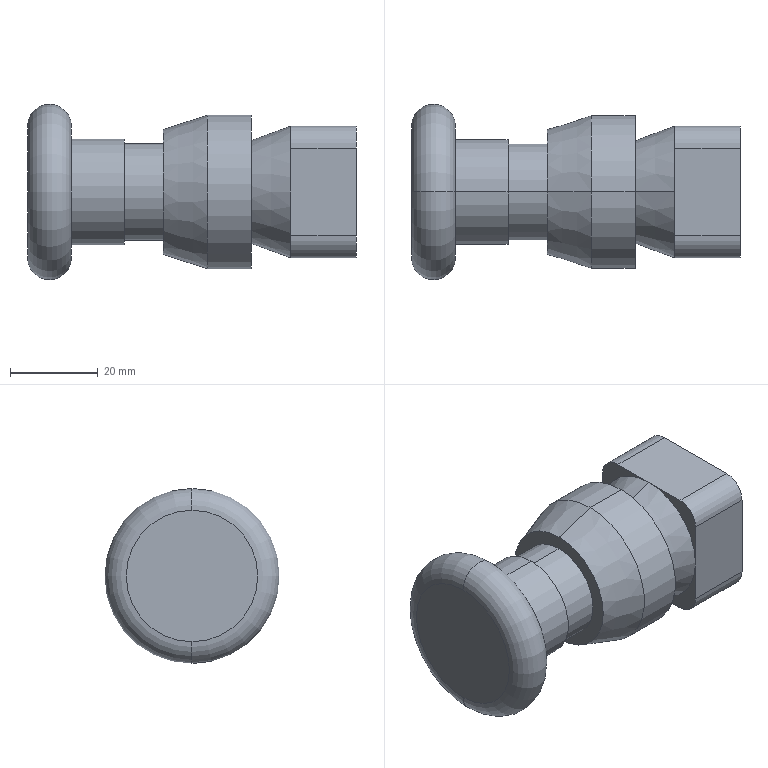Part | SolidWorks | features BaseBody 1 | 1 solid | 30 faces | box 75 x 40 x 40 mm | volume 55961 mm3 | plane 14 | cylinder 10 | cone 4 | torus 2 | commonest cylinder face diameters 10 x4 22 x2 24 x2 35 x2
STEP:
#1=CARTESIAN_POINT('',(3.054,-15.123,17.5));
#2=VERTEX_POINT('',#1);
#3=CARTESIAN_POINT('',(3.054,-15.123,-17.5));
#4=VERTEX_POINT('',#3);
#5=CARTESIAN_POINT('',(3.054,-15.123,0.));
#6=DIRECTION('',(-1.,0.,0.));
#7=DIRECTION('',(0.,0.,1.));
#8=AXIS2_PLACEMENT_3D('',#5,#6,#7);
#9=CIRCLE('',#8,17.5);
#10=EDGE_CURVE('',#2,#4,#9,.T.);
#11=ORIENTED_EDGE('',*,*,#10,.F.);
#12=CARTESIAN_POINT('',(13.054,-15.123,17.5));
#13=VERTEX_POINT('',#12);
#14=CARTESIAN_POINT('',(3.054,-15.123,17.5));
#15=DIRECTION('',(1.,0.,0.));
#16=VECTOR('',#15,1000.);
#17=LINE('',#14,#16);
#18=EDGE_CURVE('',#2,#13,#17,.T.);
#19=ORIENTED_EDGE('',*,*,#18,.T.);
#20=CARTESIAN_POINT('',(13.054,-15.123,-17.5));
#21=VERTEX_POINT('',#20);
#22=CARTESIAN_POINT('',(13.054,-15.123,0.));
#23=DIRECTION('',(1.,0.,0.));
#24=DIRECTION('',(0.,0.,-1.));
#25=AXIS2_PLACEMENT_3D('',#22,#23,#24);
#26=CIRCLE('',#25,17.5);
#27=EDGE_CURVE('',#21,#13,#26,.T.);
#28=ORIENTED_EDGE('',*,*,#27,.F.);
#29=CARTESIAN_POINT('',(3.054,-15.123,-17.5));
#30=DIRECTION('',(1.,0.,0.));
#31=VECTOR('',#30,1000.);
#32=LINE('',#29,#31);
#33=EDGE_CURVE('',#4,#21,#32,.T.);
#34=ORIENTED_EDGE('',*,*,#33,.F.);
#35=EDGE_LOOP('',(#11,#19,#28,#34));
#36=FACE_OUTER_BOUND('',#35,.T.);
#37=CARTESIAN_POINT('',(3.054,-15.123,0.));
#38=DIRECTION('',(1.,0.,0.));
#39=DIRECTION('',(0.,0.,-1.));
#40=AXIS2_PLACEMENT_3D('',#37,#38,#39);
#41=CYLINDRICAL_SURFACE('',#40,17.5);
#42=ADVANCED_FACE('',(#36),#41,.T.);
#43=CARTESIAN_POINT('',(13.054,-15.123,11.724));
#44=VERTEX_POINT('',#43);
#45=CARTESIAN_POINT('',(13.054,-15.123,-11.724));
#46=VERTEX_POINT('',#45);
#47=CARTESIAN_POINT('',(13.054,-15.123,0.));
#48=DIRECTION('',(1.,0.,0.));
#49=DIRECTION('',(0.,0.,-1.));
#50=AXIS2_PLACEMENT_3D('',#47,#48,#49);
#51=CIRCLE('',#50,11.724);
#52=EDGE_CURVE('',#44,#46,#51,.T.);
#53=ORIENTED_EDGE('',*,*,#52,.T.);
#54=CARTESIAN_POINT('',(22.054,-15.123,-15.));
#55=VERTEX_POINT('',#54);
#56=CARTESIAN_POINT('',(22.054,-15.123,-15.));
#57=DIRECTION('',(0.9397,0.,-0.342));
#58=VECTOR('',#57,1000.);
#59=LINE('',#56,#58);
#60=EDGE_CURVE('',#46,#55,#59,.T.);
#61=ORIENTED_EDGE('',*,*,#60,.T.);
#62=CARTESIAN_POINT('',(22.054,-30.123,0.));
#63=VERTEX_POINT('',#62);
#64=CARTESIAN_POINT('',(22.054,-15.123,0.));
#65=DIRECTION('',(-1.,0.,0.));
#66=DIRECTION('',(0.,0.,1.));
#67=AXIS2_PLACEMENT_3D('',#64,#65,#66);
#68=CIRCLE('',#67,15.);
#69=EDGE_CURVE('',#55,#63,#68,.T.);
#70=ORIENTED_EDGE('',*,*,#69,.T.);
#71=CARTESIAN_POINT('',(22.054,-15.123,15.));
#72=VERTEX_POINT('',#71);
#73=CARTESIAN_POINT('',(22.054,-15.123,0.));
#74=DIRECTION('',(-1.,0.,0.));
#75=DIRECTION('',(0.,0.,1.));
#76=AXIS2_PLACEMENT_3D('',#73,#74,#75);
#77=CIRCLE('',#76,15.);
#78=EDGE_CURVE('',#63,#72,#77,.T.);
#79=ORIENTED_EDGE('',*,*,#78,.T.);
#80=CARTESIAN_POINT('',(22.054,-15.123,15.));
#81=DIRECTION('',(0.9397,0.,0.342));
#82=VECTOR('',#81,1000.);
#83=LINE('',#80,#82);
#84=EDGE_CURVE('',#44,#72,#83,.T.);
#85=ORIENTED_EDGE('',*,*,#84,.F.);
#86=EDGE_LOOP('',(#53,#61,#70,#79,#85));
#87=FACE_OUTER_BOUND('',#86,.T.);
#88=CARTESIAN_POINT('',(22.054,-15.123,0.));
#89=DIRECTION('',(1.,0.,0.));
#90=DIRECTION('',(0.,0.,1.));
#91=AXIS2_PLACEMENT_3D('',#88,#89,#90);
#92=CONICAL_SURFACE('',#91,15.,0.3491);
#93=ADVANCED_FACE('',(#87),#92,.T.);
#94=CARTESIAN_POINT('',(-6.946,-15.123,-14.251));
#95=VERTEX_POINT('',#94);
#96=CARTESIAN_POINT('',(-6.946,-15.123,14.251));
#97=VERTEX_POINT('',#96);
#98=CARTESIAN_POINT('',(-6.946,-15.123,0.));
#99=DIRECTION('',(-1.,0.,0.));
#100=DIRECTION('',(0.,0.,1.));
#101=AXIS2_PLACEMENT_3D('',#98,#99,#100);
#102=CIRCLE('',#101,14.251);
#103=EDGE_CURVE('',#95,#97,#102,.T.);
#104=ORIENTED_EDGE('',*,*,#103,.F.);
#105=CARTESIAN_POINT('',(3.054,-15.123,-17.5));
#106=DIRECTION('',(0.9511,0.,-0.309));
#107=VECTOR('',#106,1000.);
#108=LINE('',#105,#107);
#109=EDGE_CURVE('',#95,#4,#108,.T.);
#110=ORIENTED_EDGE('',*,*,#109,.T.);
#111=CARTESIAN_POINT('',(3.054,-15.123,0.));
#112=DIRECTION('',(-1.,0.,0.));
#113=DIRECTION('',(0.,0.,1.));
#114=AXIS2_PLACEMENT_3D('',#111,#112,#113);
#115=CIRCLE('',#114,17.5);
#116=EDGE_CURVE('',#4,#2,#115,.T.);
#117=ORIENTED_EDGE('',*,*,#116,.T.);
#118=CARTESIAN_POINT('',(3.054,-15.123,17.5));
#119=DIRECTION('',(0.9511,0.,0.309));
#120=VECTOR('',#119,1000.);
#121=LINE('',#118,#120);
#122=EDGE_CURVE('',#97,#2,#121,.T.);
#123=ORIENTED_EDGE('',*,*,#122,.F.);
#124=EDGE_LOOP('',(#104,#110,#117,#123));
#125=FACE_OUTER_BOUND('',#124,.T.);
#126=CARTESIAN_POINT('',(3.054,-15.123,0.));
#127=DIRECTION('',(1.,0.,0.));
#128=DIRECTION('',(0.,0.,1.));
#129=AXIS2_PLACEMENT_3D('',#126,#127,#128);
#130=CONICAL_SURFACE('',#129,17.5,0.3142);
#131=ADVANCED_FACE('',(#125),#130,.T.);
#132=CARTESIAN_POINT('',(-27.946,-15.123,15.));
#133=VERTEX_POINT('',#132);
#134=CARTESIAN_POINT('',(-27.946,-15.123,-15.));
#135=VERTEX_POINT('',#134);
#136=CARTESIAN_POINT('',(-27.946,-15.123,0.));
#137=DIRECTION('',(-1.,0.,0.));
#138=DIRECTION('',(0.,0.,1.));
#139=AXIS2_PLACEMENT_3D('',#136,#137,#138);
#140=CIRCLE('',#139,15.);
#141=EDGE_CURVE('',#133,#135,#140,.T.);
#142=ORIENTED_EDGE('',*,*,#141,.T.);
#143=CARTESIAN_POINT('',(-37.946,-15.123,-15.));
#144=VERTEX_POINT('',#143);
#145=CARTESIAN_POINT('',(-32.946,-15.123,-15.));
#146=DIRECTION('',(0.,1.,0.));
#147=DIRECTION('',(0.,0.,1.));
#148=AXIS2_PLACEMENT_3D('',#145,#146,#147);
#149=CIRCLE('',#148,5.);
#150=EDGE_CURVE('',#135,#144,#149,.T.);
#151=ORIENTED_EDGE('',*,*,#150,.T.);
#152=CARTESIAN_POINT('',(-37.946,-15.123,15.));
#153=VERTEX_POINT('',#152);
#154=CARTESIAN_POINT('',(-37.946,-15.123,0.));
#155=DIRECTION('',(-1.,0.,0.));
#156=DIRECTION('',(0.,0.,1.));
#157=AXIS2_PLACEMENT_3D('',#154,#155,#156);
#158=CIRCLE('',#157,15.);
#159=EDGE_CURVE('',#153,#144,#158,.T.);
#160=ORIENTED_EDGE('',*,*,#159,.F.);
#161=CARTESIAN_POINT('',(-32.946,-15.123,15.));
#162=DIRECTION('',(0.,-1.,0.));
#163=DIRECTION('',(0.,0.,-1.));
#164=AXIS2_PLACEMENT_3D('',#161,#162,#163);
#165=CIRCLE('',#164,5.);
#166=EDGE_CURVE('',#133,#153,#165,.T.);
#167=ORIENTED_EDGE('',*,*,#166,.F.);
#168=EDGE_LOOP('',(#142,#151,#160,#167));
#169=FACE_OUTER_BOUND('',#168,.T.);
#170=CARTESIAN_POINT('',(-32.946,-15.123,0.));
#171=DIRECTION('',(-1.,0.,0.));
#172=DIRECTION('',(0.,0.,1.));
#173=AXIS2_PLACEMENT_3D('',#170,#171,#172);
#174=TOROIDAL_SURFACE('',#173,15.,5.);
#175=ADVANCED_FACE('',(#169),#174,.T.);
#176=CARTESIAN_POINT('',(-15.946,-15.123,12.));
#177=VERTEX_POINT('',#176);
#178=CARTESIAN_POINT('',(-15.946,-15.123,-12.));
#179=VERTEX_POINT('',#178);
#180=CARTESIAN_POINT('',(-15.946,-15.123,0.));
#181=DIRECTION('',(-1.,0.,0.));
#182=DIRECTION('',(0.,0.,1.));
#183=AXIS2_PLACEMENT_3D('',#180,#181,#182);
#184=CIRCLE('',#183,12.);
#185=EDGE_CURVE('',#177,#179,#184,.T.);
#186=ORIENTED_EDGE('',*,*,#185,.T.);
#187=CARTESIAN_POINT('',(-27.946,-15.123,-12.));
#188=VERTEX_POINT('',#187);
#189=CARTESIAN_POINT('',(-37.946,-15.123,-12.));
#190=DIRECTION('',(-1.,0.,0.));
#191=VECTOR('',#190,1000.);
#192=LINE('',#189,#191);
#193=EDGE_CURVE('',#179,#188,#192,.T.);
#194=ORIENTED_EDGE('',*,*,#193,.T.);
#195=CARTESIAN_POINT('',(-27.946,-15.123,12.));
#196=VERTEX_POINT('',#195);
#197=CARTESIAN_POINT('',(-27.946,-15.123,0.));
#198=DIRECTION('',(-1.,0.,0.));
#199=DIRECTION('',(0.,0.,1.));
#200=AXIS2_PLACEMENT_3D('',#197,#198,#199);
#201=CIRCLE('',#200,12.);
#202=EDGE_CURVE('',#196,#188,#201,.T.);
#203=ORIENTED_EDGE('',*,*,#202,.F.);
#204=CARTESIAN_POINT('',(-37.946,-15.123,12.));
#205=DIRECTION('',(-1.,0.,0.));
#206=VECTOR('',#205,1000.);
#207=LINE('',#204,#206);
#208=EDGE_CURVE('',#177,#196,#207,.T.);
#209=ORIENTED_EDGE('',*,*,#208,.F.);
#210=EDGE_LOOP('',(#186,#194,#203,#209));
#211=FACE_OUTER_BOUND('',#210,.T.);
#212=CARTESIAN_POINT('',(-37.946,-15.123,0.));
#213=DIRECTION('',(-1.,0.,0.));
#214=DIRECTION('',(0.,0.,1.));
#215=AXIS2_PLACEMENT_3D('',#212,#213,#214);
#216=CYLINDRICAL_SURFACE('',#215,12.);
#217=ADVANCED_FACE('',(#211),#216,.T.);
#218=CARTESIAN_POINT('',(-6.946,-15.123,11.));
#219=VERTEX_POINT('',#218);
#220=CARTESIAN_POINT('',(-6.946,-15.123,-11.));
#221=VERTEX_POINT('',#220);
#222=CARTESIAN_POINT('',(-6.946,-15.123,0.));
#223=DIRECTION('',(-1.,0.,0.));
#224=DIRECTION('',(0.,0.,1.));
#225=AXIS2_PLACEMENT_3D('',#222,#223,#224);
#226=CIRCLE('',#225,11.);
#227=EDGE_CURVE('',#219,#221,#226,.T.);
#228=ORIENTED_EDGE('',*,*,#227,.T.);
#229=CARTESIAN_POINT('',(-15.946,-15.123,-11.));
#230=VERTEX_POINT('',#229);
#231=CARTESIAN_POINT('',(-37.946,-15.123,-11.));
#232=DIRECTION('',(-1.,0.,0.));
#233=VECTOR('',#232,1000.);
#234=LINE('',#231,#233);
#235=EDGE_CURVE('',#221,#230,#234,.T.);
#236=ORIENTED_EDGE('',*,*,#235,.T.);
#237=CARTESIAN_POINT('',(-15.946,-15.123,11.));
#238=VERTEX_POINT('',#237);
#239=CARTESIAN_POINT('',(-15.946,-15.123,0.));
#240=DIRECTION('',(-1.,0.,0.));
#241=DIRECTION('',(0.,0.,1.));
#242=AXIS2_PLACEMENT_3D('',#239,#240,#241);
#243=CIRCLE('',#242,11.);
#244=EDGE_CURVE('',#238,#230,#243,.T.);
#245=ORIENTED_EDGE('',*,*,#244,.F.);
#246=CARTESIAN_POINT('',(-37.946,-15.123,11.));
#247=DIRECTION('',(-1.,0.,0.));
#248=VECTOR('',#247,1000.);
#249=LINE('',#246,#248);
#250=EDGE_CURVE('',#219,#238,#249,.T.);
#251=ORIENTED_EDGE('',*,*,#250,.F.);
#252=EDGE_LOOP('',(#228,#236,#245,#251));
#253=FACE_OUTER_BOUND('',#252,.T.);
#254=CARTESIAN_POINT('',(-37.946,-15.123,0.));
#255=DIRECTION('',(-1.,0.,0.));
#256=DIRECTION('',(0.,0.,1.));
#257=AXIS2_PLACEMENT_3D('',#254,#255,#256);
#258=CYLINDRICAL_SURFACE('',#257,11.);
#259=ADVANCED_FACE('',(#253),#258,.T.);
#260=CARTESIAN_POINT('',(22.054,-0.1235,-10.));
#261=VERTEX_POINT('',#260);
#262=CARTESIAN_POINT('',(22.054,-5.123,-15.));
#263=VERTEX_POINT('',#262);
#264=CARTESIAN_POINT('',(22.054,-5.123,-10.));
#265=DIRECTION('',(-1.,0.,0.));
#266=DIRECTION('',(0.,0.,-1.));
#267=AXIS2_PLACEMENT_3D('',#264,#265,#266);
#268=CIRCLE('',#267,5.);
#269=EDGE_CURVE('',#261,#263,#268,.T.);
#270=ORIENTED_EDGE('',*,*,#269,.F.);
#271=CARTESIAN_POINT('',(37.054,-0.1235,-10.));
#272=VERTEX_POINT('',#271);
#273=CARTESIAN_POINT('',(22.054,-0.1235,-10.));
#274=DIRECTION('',(-1.,0.,0.));
#275=VECTOR('',#274,1000.);
#276=LINE('',#273,#275);
#277=EDGE_CURVE('',#272,#261,#276,.T.);
#278=ORIENTED_EDGE('',*,*,#277,.F.);
#279=CARTESIAN_POINT('',(37.054,-5.123,-15.));
#280=VERTEX_POINT('',#279);
#281=CARTESIAN_POINT('',(37.054,-5.123,-10.));
#282=DIRECTION('',(1.,0.,0.));
#283=DIRECTION('',(0.,0.,-1.));
#284=AXIS2_PLACEMENT_3D('',#281,#282,#283);
#285=CIRCLE('',#284,5.);
#286=EDGE_CURVE('',#280,#272,#285,.T.);
#287=ORIENTED_EDGE('',*,*,#286,.F.);
#288=CARTESIAN_POINT('',(22.054,-5.123,-15.));
#289=DIRECTION('',(1.,0.,0.));
#290=VECTOR('',#289,1000.);
#291=LINE('',#288,#290);
#292=EDGE_CURVE('',#263,#280,#291,.T.);
#293=ORIENTED_EDGE('',*,*,#292,.F.);
#294=EDGE_LOOP('',(#270,#278,#287,#293));
#295=FACE_OUTER_BOUND('',#294,.T.);
#296=CARTESIAN_POINT('',(22.054,-5.123,-10.));
#297=DIRECTION('',(1.,0.,0.));
#298=DIRECTION('',(0.,0.,-1.));
#299=AXIS2_PLACEMENT_3D('',#296,#297,#298);
#300=CYLINDRICAL_SURFACE('',#299,5.);
#301=ADVANCED_FACE('',(#295),#300,.T.);
#302=CARTESIAN_POINT('',(22.054,-25.123,-15.));
#303=VERTEX_POINT('',#302);
#304=CARTESIAN_POINT('',(22.054,-30.123,-10.));
#305=VERTEX_POINT('',#304);
#306=CARTESIAN_POINT('',(22.054,-25.123,-10.));
#307=DIRECTION('',(-1.,0.,0.));
#308=DIRECTION('',(0.,0.,-1.));
#309=AXIS2_PLACEMENT_3D('',#306,#307,#308);
#310=CIRCLE('',#309,5.);
#311=EDGE_CURVE('',#303,#305,#310,.T.);
#312=ORIENTED_EDGE('',*,*,#311,.F.);
#313=CARTESIAN_POINT('',(37.054,-25.123,-15.));
#314=VERTEX_POINT('',#313);
#315=CARTESIAN_POINT('',(22.054,-25.123,-15.));
#316=DIRECTION('',(-1.,0.,0.));
#317=VECTOR('',#316,1000.);
#318=LINE('',#315,#317);
#319=EDGE_CURVE('',#314,#303,#318,.T.);
#320=ORIENTED_EDGE('',*,*,#319,.F.);
#321=CARTESIAN_POINT('',(37.054,-30.123,-10.));
#322=VERTEX_POINT('',#321);
#323=CARTESIAN_POINT('',(37.054,-25.123,-10.));
#324=DIRECTION('',(1.,0.,0.));
#325=DIRECTION('',(0.,0.,-1.));
#326=AXIS2_PLACEMENT_3D('',#323,#324,#325);
#327=CIRCLE('',#326,5.);
#328=EDGE_CURVE('',#322,#314,#327,.T.);
#329=ORIENTED_EDGE('',*,*,#328,.F.);
#330=CARTESIAN_POINT('',(22.054,-30.123,-10.));
#331=DIRECTION('',(1.,0.,0.));
#332=VECTOR('',#331,1000.);
#333=LINE('',#330,#332);
#334=EDGE_CURVE('',#305,#322,#333,.T.);
#335=ORIENTED_EDGE('',*,*,#334,.F.);
#336=EDGE_LOOP('',(#312,#320,#329,#335));
#337=FACE_OUTER_BOUND('',#336,.T.);
#338=CARTESIAN_POINT('',(22.054,-25.123,-10.));
#339=DIRECTION('',(1.,0.,0.));
#340=DIRECTION('',(0.,0.,-1.));
#341=AXIS2_PLACEMENT_3D('',#338,#339,#340);
#342=CYLINDRICAL_SURFACE('',#341,5.);
#343=ADVANCED_FACE('',(#337),#342,.T.);
#344=CARTESIAN_POINT('',(22.054,-5.123,15.));
#345=VERTEX_POINT('',#344);
#346=CARTESIAN_POINT('',(22.054,-0.1235,10.));
#347=VERTEX_POINT('',#346);
#348=CARTESIAN_POINT('',(22.054,-5.123,10.));
#349=DIRECTION('',(-1.,0.,0.));
#350=DIRECTION('',(0.,0.,-1.));
#351=AXIS2_PLACEMENT_3D('',#348,#349,#350);
#352=CIRCLE('',#351,5.);
#353=EDGE_CURVE('',#345,#347,#352,.T.);
#354=ORIENTED_EDGE('',*,*,#353,.F.);
#355=CARTESIAN_POINT('',(37.054,-5.123,15.));
#356=VERTEX_POINT('',#355);
#357=CARTESIAN_POINT('',(22.054,-5.123,15.));
#358=DIRECTION('',(-1.,0.,0.));
#359=VECTOR('',#358,1000.);
#360=LINE('',#357,#359);
#361=EDGE_CURVE('',#356,#345,#360,.T.);
#362=ORIENTED_EDGE('',*,*,#361,.F.);
#363=CARTESIAN_POINT('',(37.054,-0.1235,10.));
#364=VERTEX_POINT('',#363);
#365=CARTESIAN_POINT('',(37.054,-5.123,10.));
#366=DIRECTION('',(1.,0.,0.));
#367=DIRECTION('',(0.,0.,-1.));
#368=AXIS2_PLACEMENT_3D('',#365,#366,#367);
#369=CIRCLE('',#368,5.);
#370=EDGE_CURVE('',#364,#356,#369,.T.);
#371=ORIENTED_EDGE('',*,*,#370,.F.);
#372=CARTESIAN_POINT('',(22.054,-0.1235,10.));
#373=DIRECTION('',(1.,0.,0.));
#374=VECTOR('',#373,1000.);
#375=LINE('',#372,#374);
#376=EDGE_CURVE('',#347,#364,#375,.T.);
#377=ORIENTED_EDGE('',*,*,#376,.F.);
#378=EDGE_LOOP('',(#354,#362,#371,#377));
#379=FACE_OUTER_BOUND('',#378,.T.);
#380=CARTESIAN_POINT('',(22.054,-5.123,10.));
#381=DIRECTION('',(1.,0.,0.));
#382=DIRECTION('',(0.,0.,-1.));
#383=AXIS2_PLACEMENT_3D('',#380,#381,#382);
#384=CYLINDRICAL_SURFACE('',#383,5.);
#385=ADVANCED_FACE('',(#379),#384,.T.);
#386=CARTESIAN_POINT('',(22.054,-30.123,10.));
#387=VERTEX_POINT('',#386);
#388=CARTESIAN_POINT('',(22.054,-25.123,15.));
#389=VERTEX_POINT('',#388);
#390=CARTESIAN_POINT('',(22.054,-25.123,10.));
#391=DIRECTION('',(-1.,0.,0.));
#392=DIRECTION('',(0.,0.,-1.));
#393=AXIS2_PLACEMENT_3D('',#390,#391,#392);
#394=CIRCLE('',#393,5.);
#395=EDGE_CURVE('',#387,#389,#394,.T.);
#396=ORIENTED_EDGE('',*,*,#395,.F.);
#397=CARTESIAN_POINT('',(37.054,-30.123,10.));
#398=VERTEX_POINT('',#397);
#399=CARTESIAN_POINT('',(22.054,-30.123,10.));
#400=DIRECTION('',(-1.,0.,0.));
#401=VECTOR('',#400,1000.);
#402=LINE('',#399,#401);
#403=EDGE_CURVE('',#398,#387,#402,.T.);
#404=ORIENTED_EDGE('',*,*,#403,.F.);
#405=CARTESIAN_POINT('',(37.054,-25.123,15.));
#406=VERTEX_POINT('',#405);
#407=CARTESIAN_POINT('',(37.054,-25.123,10.));
#408=DIRECTION('',(1.,0.,0.));
#409=DIRECTION('',(0.,0.,-1.));
#410=AXIS2_PLACEMENT_3D('',#407,#408,#409);
#411=CIRCLE('',#410,5.);
#412=EDGE_CURVE('',#406,#398,#411,.T.);
#413=ORIENTED_EDGE('',*,*,#412,.F.);
#414=CARTESIAN_POINT('',(22.054,-25.123,15.));
#415=DIRECTION('',(1.,0.,0.));
#416=VECTOR('',#415,1000.);
#417=LINE('',#414,#416);
#418=EDGE_CURVE('',#389,#406,#417,.T.);
#419=ORIENTED_EDGE('',*,*,#418,.F.);
#420=EDGE_LOOP('',(#396,#404,#413,#419));
#421=FACE_OUTER_BOUND('',#420,.T.);
#422=CARTESIAN_POINT('',(22.054,-25.123,10.));
#423=DIRECTION('',(1.,0.,0.));
#424=DIRECTION('',(0.,0.,-1.));
#425=AXIS2_PLACEMENT_3D('',#422,#423,#424);
#426=CYLINDRICAL_SURFACE('',#425,5.);
#427=ADVANCED_FACE('',(#421),#426,.T.);
#428=CARTESIAN_POINT('',(37.054,-30.123,15.));
#429=DIRECTION('',(0.,-1.,0.));
#430=VECTOR('',#429,1000.);
#431=LINE('',#428,#430);
#432=EDGE_CURVE('',#356,#406,#431,.T.);
#433=ORIENTED_EDGE('',*,*,#432,.T.);
#434=ORIENTED_EDGE('',*,*,#412,.T.);
#435=CARTESIAN_POINT('',(37.054,-30.123,-15.));
#436=DIRECTION('',(0.,0.,-1.));
#437=VECTOR('',#436,1000.);
#438=LINE('',#435,#437);
#439=EDGE_CURVE('',#398,#322,#438,.T.);
#440=ORIENTED_EDGE('',*,*,#439,.T.);
#441=ORIENTED_EDGE('',*,*,#328,.T.);
#442=CARTESIAN_POINT('',(37.054,-30.123,-15.));
#443=DIRECTION('',(0.,1.,0.));
#444=VECTOR('',#443,1000.);
#445=LINE('',#442,#444);
#446=EDGE_CURVE('',#314,#280,#445,.T.);
#447=ORIENTED_EDGE('',*,*,#446,.T.);
#448=ORIENTED_EDGE('',*,*,#286,.T.);
#449=CARTESIAN_POINT('',(37.054,-0.1235,-15.));
#450=DIRECTION('',(0.,0.,1.));
#451=VECTOR('',#450,1000.);
#452=LINE('',#449,#451);
#453=EDGE_CURVE('',#272,#364,#452,.T.);
#454=ORIENTED_EDGE('',*,*,#453,.T.);
#455=ORIENTED_EDGE('',*,*,#370,.T.);
#456=EDGE_LOOP('',(#433,#434,#440,#441,#447,#448,#454,#455));
#457=FACE_OUTER_BOUND('',#456,.T.);
#458=CARTESIAN_POINT('',(37.054,-15.123,0.));
#459=DIRECTION('',(1.,0.,0.));
#460=DIRECTION('',(0.,1.,0.));
#461=AXIS2_PLACEMENT_3D('',#458,#459,#460);
#462=PLANE('',#461);
#463=ADVANCED_FACE('',(#457),#462,.T.);
#464=CARTESIAN_POINT('',(22.054,-30.123,-15.));
#465=DIRECTION('',(0.,1.,0.));
#466=VECTOR('',#465,1000.);
#467=LINE('',#464,#466);
#468=EDGE_CURVE('',#303,#55,#467,.T.);
#469=ORIENTED_EDGE('',*,*,#468,.F.);
#470=ORIENTED_EDGE('',*,*,#311,.T.);
#471=CARTESIAN_POINT('',(22.054,-30.123,-15.));
#472=DIRECTION('',(0.,0.,-1.));
#473=VECTOR('',#472,1000.);
#474=LINE('',#471,#473);
#475=EDGE_CURVE('',#63,#305,#474,.T.);
#476=ORIENTED_EDGE('',*,*,#475,.F.);
#477=ORIENTED_EDGE('',*,*,#69,.F.);
#478=EDGE_LOOP('',(#469,#470,#476,#477));
#479=FACE_OUTER_BOUND('',#478,.T.);
#480=CARTESIAN_POINT('',(22.054,0.,0.));
#481=DIRECTION('',(1.,0.,0.));
#482=DIRECTION('',(0.,1.,0.));
#483=AXIS2_PLACEMENT_3D('',#480,#481,#482);
#484=PLANE('',#483);
#485=ADVANCED_FACE('',(#479),#484,.F.);
#486=CARTESIAN_POINT('',(22.054,-30.123,-15.));
#487=DIRECTION('',(0.,0.,-1.));
#488=VECTOR('',#487,1000.);
#489=LINE('',#486,#488);
#490=EDGE_CURVE('',#387,#63,#489,.T.);
#491=ORIENTED_EDGE('',*,*,#490,.F.);
#492=ORIENTED_EDGE('',*,*,#395,.T.);
#493=CARTESIAN_POINT('',(22.054,-30.123,15.));
#494=DIRECTION('',(0.,-1.,0.));
#495=VECTOR('',#494,1000.);
#496=LINE('',#493,#495);
#497=EDGE_CURVE('',#72,#389,#496,.T.);
#498=ORIENTED_EDGE('',*,*,#497,.F.);
#499=ORIENTED_EDGE('',*,*,#78,.F.);
#500=EDGE_LOOP('',(#491,#492,#498,#499));
#501=FACE_OUTER_BOUND('',#500,.T.);
#502=CARTESIAN_POINT('',(22.054,0.,0.));
#503=DIRECTION('',(1.,0.,0.));
#504=DIRECTION('',(0.,1.,0.));
#505=AXIS2_PLACEMENT_3D('',#502,#503,#504);
#506=PLANE('',#505);
#507=ADVANCED_FACE('',(#501),#506,.F.);
#508=CARTESIAN_POINT('',(22.054,-30.123,15.));
#509=DIRECTION('',(0.,-1.,0.));
#510=VECTOR('',#509,1000.);
#511=LINE('',#508,#510);
#512=EDGE_CURVE('',#345,#72,#511,.T.);
#513=ORIENTED_EDGE('',*,*,#512,.F.);
#514=ORIENTED_EDGE('',*,*,#353,.T.);
#515=CARTESIAN_POINT('',(22.054,-0.1235,0.));
#516=VERTEX_POINT('',#515);
#517=CARTESIAN_POINT('',(22.054,-0.1235,-15.));
#518=DIRECTION('',(0.,0.,1.));
#519=VECTOR('',#518,1000.);
#520=LINE('',#517,#519);
#521=EDGE_CURVE('',#516,#347,#520,.T.);
#522=ORIENTED_EDGE('',*,*,#521,.F.);
#523=CARTESIAN_POINT('',(22.054,-15.123,0.));
#524=DIRECTION('',(-1.,0.,0.));
#525=DIRECTION('',(0.,0.,1.));
#526=AXIS2_PLACEMENT_3D('',#523,#524,#525);
#527=CIRCLE('',#526,15.);
#528=EDGE_CURVE('',#72,#516,#527,.T.);
#529=ORIENTED_EDGE('',*,*,#528,.F.);
#530=EDGE_LOOP('',(#513,#514,#522,#529));
#531=FACE_OUTER_BOUND('',#530,.T.);
#532=CARTESIAN_POINT('',(22.054,0.,0.));
#533=DIRECTION('',(1.,0.,0.));
#534=DIRECTION('',(0.,1.,0.));
#535=AXIS2_PLACEMENT_3D('',#532,#533,#534);
#536=PLANE('',#535);
#537=ADVANCED_FACE('',(#531),#536,.F.);
#538=CARTESIAN_POINT('',(22.054,-0.1235,-15.));
#539=DIRECTION('',(0.,0.,1.));
#540=VECTOR('',#539,1000.);
#541=LINE('',#538,#540);
#542=EDGE_CURVE('',#261,#516,#541,.T.);
#543=ORIENTED_EDGE('',*,*,#542,.F.);
#544=ORIENTED_EDGE('',*,*,#269,.T.);
#545=CARTESIAN_POINT('',(22.054,-30.123,-15.));
#546=DIRECTION('',(0.,1.,0.));
#547=VECTOR('',#546,1000.);
#548=LINE('',#545,#547);
#549=EDGE_CURVE('',#55,#263,#548,.T.);
#550=ORIENTED_EDGE('',*,*,#549,.F.);
#551=CARTESIAN_POINT('',(22.054,-15.123,0.));
#552=DIRECTION('',(-1.,0.,0.));
#553=DIRECTION('',(0.,0.,1.));
#554=AXIS2_PLACEMENT_3D('',#551,#552,#553);
#555=CIRCLE('',#554,15.);
#556=EDGE_CURVE('',#516,#55,#555,.T.);
#557=ORIENTED_EDGE('',*,*,#556,.F.);
#558=EDGE_LOOP('',(#543,#544,#550,#557));
#559=FACE_OUTER_BOUND('',#558,.T.);
#560=CARTESIAN_POINT('',(22.054,0.,0.));
#561=DIRECTION('',(1.,0.,0.));
#562=DIRECTION('',(0.,1.,0.));
#563=AXIS2_PLACEMENT_3D('',#560,#561,#562);
#564=PLANE('',#563);
#565=ADVANCED_FACE('',(#559),#564,.F.);
#566=ORIENTED_EDGE('',*,*,#521,.T.);
#567=ORIENTED_EDGE('',*,*,#376,.T.);
#568=ORIENTED_EDGE('',*,*,#453,.F.);
#569=ORIENTED_EDGE('',*,*,#277,.T.);
#570=ORIENTED_EDGE('',*,*,#542,.T.);
#571=EDGE_LOOP('',(#566,#567,#568,#569,#570));
#572=FACE_OUTER_BOUND('',#571,.T.);
#573=CARTESIAN_POINT('',(22.054,-0.1235,-15.));
#574=DIRECTION('',(0.,1.,0.));
#575=DIRECTION('',(0.,0.,-1.));
#576=AXIS2_PLACEMENT_3D('',#573,#574,#575);
#577=PLANE('',#576);
#578=ADVANCED_FACE('',(#572),#577,.T.);
#579=ORIENTED_EDGE('',*,*,#497,.T.);
#580=ORIENTED_EDGE('',*,*,#418,.T.);
#581=ORIENTED_EDGE('',*,*,#432,.F.);
#582=ORIENTED_EDGE('',*,*,#361,.T.);
#583=ORIENTED_EDGE('',*,*,#512,.T.);
#584=EDGE_LOOP('',(#579,#580,#581,#582,#583));
#585=FACE_OUTER_BOUND('',#584,.T.);
#586=CARTESIAN_POINT('',(22.054,-30.123,15.));
#587=DIRECTION('',(0.,0.,1.));
#588=DIRECTION('',(1.,0.,0.));
#589=AXIS2_PLACEMENT_3D('',#586,#587,#588);
#590=PLANE('',#589);
#591=ADVANCED_FACE('',(#585),#590,.T.);
#592=ORIENTED_EDGE('',*,*,#439,.F.);
#593=ORIENTED_EDGE('',*,*,#403,.T.);
#594=ORIENTED_EDGE('',*,*,#490,.T.);
#595=ORIENTED_EDGE('',*,*,#475,.T.);
#596=ORIENTED_EDGE('',*,*,#334,.T.);
#597=EDGE_LOOP('',(#592,#593,#594,#595,#596));
#598=FACE_OUTER_BOUND('',#597,.T.);
#599=CARTESIAN_POINT('',(22.054,-30.123,-15.));
#600=DIRECTION('',(0.,-1.,0.));
#601=DIRECTION('',(0.,0.,-1.));
#602=AXIS2_PLACEMENT_3D('',#599,#600,#601);
#603=PLANE('',#602);
#604=ADVANCED_FACE('',(#598),#603,.T.);
#605=ORIENTED_EDGE('',*,*,#446,.F.);
#606=ORIENTED_EDGE('',*,*,#319,.T.);
#607=ORIENTED_EDGE('',*,*,#468,.T.);
#608=ORIENTED_EDGE('',*,*,#549,.T.);
#609=ORIENTED_EDGE('',*,*,#292,.T.);
#610=EDGE_LOOP('',(#605,#606,#607,#608,#609));
#611=FACE_OUTER_BOUND('',#610,.T.);
#612=CARTESIAN_POINT('',(22.054,-30.123,-15.));
#613=DIRECTION('',(0.,0.,-1.));
#614=DIRECTION('',(0.,-1.,0.));
#615=AXIS2_PLACEMENT_3D('',#612,#613,#614);
#616=PLANE('',#615);
#617=ADVANCED_FACE('',(#611),#616,.T.);
#618=ORIENTED_EDGE('',*,*,#52,.F.);
#619=CARTESIAN_POINT('',(13.054,-15.123,0.));
#620=DIRECTION('',(1.,0.,0.));
#621=DIRECTION('',(0.,0.,-1.));
#622=AXIS2_PLACEMENT_3D('',#619,#620,#621);
#623=CIRCLE('',#622,11.724);
#624=EDGE_CURVE('',#46,#44,#623,.T.);
#625=ORIENTED_EDGE('',*,*,#624,.F.);
#626=EDGE_LOOP('',(#618,#625));
#627=FACE_BOUND('',#626,.T.);
#628=ORIENTED_EDGE('',*,*,#27,.T.);
#629=CARTESIAN_POINT('',(13.054,-15.123,0.));
#630=DIRECTION('',(1.,0.,0.));
#631=DIRECTION('',(0.,0.,-1.));
#632=AXIS2_PLACEMENT_3D('',#629,#630,#631);
#633=CIRCLE('',#632,17.5);
#634=EDGE_CURVE('',#13,#21,#633,.T.);
#635=ORIENTED_EDGE('',*,*,#634,.T.);
#636=EDGE_LOOP('',(#628,#635));
#637=FACE_OUTER_BOUND('',#636,.T.);
#638=CARTESIAN_POINT('',(13.054,-15.123,0.));
#639=DIRECTION('',(1.,0.,0.));
#640=DIRECTION('',(0.,1.,0.));
#641=AXIS2_PLACEMENT_3D('',#638,#639,#640);
#642=PLANE('',#641);
#643=ADVANCED_FACE('',(#627,#637),#642,.T.);
#644=ORIENTED_EDGE('',*,*,#227,.F.);
#645=CARTESIAN_POINT('',(-6.946,-15.123,0.));
#646=DIRECTION('',(-1.,0.,0.));
#647=DIRECTION('',(0.,0.,1.));
#648=AXIS2_PLACEMENT_3D('',#645,#646,#647);
#649=CIRCLE('',#648,11.);
#650=EDGE_CURVE('',#221,#219,#649,.T.);
#651=ORIENTED_EDGE('',*,*,#650,.F.);
#652=EDGE_LOOP('',(#644,#651));
#653=FACE_BOUND('',#652,.T.);
#654=CARTESIAN_POINT('',(-6.946,-15.123,0.));
#655=DIRECTION('',(-1.,0.,0.));
#656=DIRECTION('',(0.,0.,1.));
#657=AXIS2_PLACEMENT_3D('',#654,#655,#656);
#658=CIRCLE('',#657,14.251);
#659=EDGE_CURVE('',#97,#95,#658,.T.);
#660=ORIENTED_EDGE('',*,*,#659,.T.);
#661=ORIENTED_EDGE('',*,*,#103,.T.);
#662=EDGE_LOOP('',(#660,#661));
#663=FACE_OUTER_BOUND('',#662,.T.);
#664=CARTESIAN_POINT('',(-6.946,-15.123,0.));
#665=DIRECTION('',(-1.,0.,0.));
#666=DIRECTION('',(0.,0.,1.));
#667=AXIS2_PLACEMENT_3D('',#664,#665,#666);
#668=PLANE('',#667);
#669=ADVANCED_FACE('',(#653,#663),#668,.T.);
#670=ORIENTED_EDGE('',*,*,#159,.T.);
#671=CARTESIAN_POINT('',(-37.946,-15.123,0.));
#672=DIRECTION('',(-1.,0.,0.));
#673=DIRECTION('',(0.,0.,1.));
#674=AXIS2_PLACEMENT_3D('',#671,#672,#673);
#675=CIRCLE('',#674,15.);
#676=EDGE_CURVE('',#144,#153,#675,.T.);
#677=ORIENTED_EDGE('',*,*,#676,.T.);
#678=EDGE_LOOP('',(#670,#677));
#679=FACE_OUTER_BOUND('',#678,.T.);
#680=CARTESIAN_POINT('',(-37.946,-3.123,0.));
#681=DIRECTION('',(1.,0.,0.));
#682=DIRECTION('',(0.,1.,0.));
#683=AXIS2_PLACEMENT_3D('',#680,#681,#682);
#684=PLANE('',#683);
#685=ADVANCED_FACE('',(#679),#684,.F.);
#686=ORIENTED_EDGE('',*,*,#202,.T.);
#687=CARTESIAN_POINT('',(-27.946,-15.123,0.));
#688=DIRECTION('',(-1.,0.,0.));
#689=DIRECTION('',(0.,0.,1.));
#690=AXIS2_PLACEMENT_3D('',#687,#688,#689);
#691=CIRCLE('',#690,12.);
#692=EDGE_CURVE('',#188,#196,#691,.T.);
#693=ORIENTED_EDGE('',*,*,#692,.T.);
#694=EDGE_LOOP('',(#686,#693));
#695=FACE_BOUND('',#694,.T.);
#696=ORIENTED_EDGE('',*,*,#141,.F.);
#697=CARTESIAN_POINT('',(-27.946,-15.123,0.));
#698=DIRECTION('',(-1.,0.,0.));
#699=DIRECTION('',(0.,0.,1.));
#700=AXIS2_PLACEMENT_3D('',#697,#698,#699);
#701=CIRCLE('',#700,15.);
#702=EDGE_CURVE('',#135,#133,#701,.T.);
#703=ORIENTED_EDGE('',*,*,#702,.F.);
#704=EDGE_LOOP('',(#696,#703));
#705=FACE_OUTER_BOUND('',#704,.T.);
#706=CARTESIAN_POINT('',(-27.946,-0.1235,0.));
#707=DIRECTION('',(-1.,0.,0.));
#708=DIRECTION('',(0.,0.,1.));
#709=AXIS2_PLACEMENT_3D('',#706,#707,#708);
#710=PLANE('',#709);
#711=ADVANCED_FACE('',(#695,#705),#710,.F.);
#712=ORIENTED_EDGE('',*,*,#244,.T.);
#713=CARTESIAN_POINT('',(-15.946,-15.123,0.));
#714=DIRECTION('',(-1.,0.,0.));
#715=DIRECTION('',(0.,0.,1.));
#716=AXIS2_PLACEMENT_3D('',#713,#714,#715);
#717=CIRCLE('',#716,11.);
#718=EDGE_CURVE('',#230,#238,#717,.T.);
#719=ORIENTED_EDGE('',*,*,#718,.T.);
#720=EDGE_LOOP('',(#712,#719));
#721=FACE_BOUND('',#720,.T.);
#722=ORIENTED_EDGE('',*,*,#185,.F.);
#723=CARTESIAN_POINT('',(-15.946,-15.123,0.));
#724=DIRECTION('',(-1.,0.,0.));
#725=DIRECTION('',(0.,0.,1.));
#726=AXIS2_PLACEMENT_3D('',#723,#724,#725);
#727=CIRCLE('',#726,12.);
#728=EDGE_CURVE('',#179,#177,#727,.T.);
#729=ORIENTED_EDGE('',*,*,#728,.F.);
#730=EDGE_LOOP('',(#722,#729));
#731=FACE_OUTER_BOUND('',#730,.T.);
#732=CARTESIAN_POINT('',(-15.946,-3.123,0.));
#733=DIRECTION('',(-1.,0.,0.));
#734=DIRECTION('',(0.,0.,1.));
#735=AXIS2_PLACEMENT_3D('',#732,#733,#734);
#736=PLANE('',#735);
#737=ADVANCED_FACE('',(#721,#731),#736,.F.);
#738=ORIENTED_EDGE('',*,*,#235,.F.);
#739=ORIENTED_EDGE('',*,*,#650,.T.);
#740=ORIENTED_EDGE('',*,*,#250,.T.);
#741=ORIENTED_EDGE('',*,*,#718,.F.);
#742=EDGE_LOOP('',(#738,#739,#740,#741));
#743=FACE_OUTER_BOUND('',#742,.T.);
#744=CARTESIAN_POINT('',(-37.946,-15.123,0.));
#745=DIRECTION('',(-1.,0.,0.));
#746=DIRECTION('',(0.,0.,1.));
#747=AXIS2_PLACEMENT_3D('',#744,#745,#746);
#748=CYLINDRICAL_SURFACE('',#747,11.);
#749=ADVANCED_FACE('',(#743),#748,.T.);
#750=ORIENTED_EDGE('',*,*,#193,.F.);
#751=ORIENTED_EDGE('',*,*,#728,.T.);
#752=ORIENTED_EDGE('',*,*,#208,.T.);
#753=ORIENTED_EDGE('',*,*,#692,.F.);
#754=EDGE_LOOP('',(#750,#751,#752,#753));
#755=FACE_OUTER_BOUND('',#754,.T.);
#756=CARTESIAN_POINT('',(-37.946,-15.123,0.));
#757=DIRECTION('',(-1.,0.,0.));
#758=DIRECTION('',(0.,0.,1.));
#759=AXIS2_PLACEMENT_3D('',#756,#757,#758);
#760=CYLINDRICAL_SURFACE('',#759,12.);
#761=ADVANCED_FACE('',(#755),#760,.T.);
#762=ORIENTED_EDGE('',*,*,#150,.F.);
#763=ORIENTED_EDGE('',*,*,#702,.T.);
#764=ORIENTED_EDGE('',*,*,#166,.T.);
#765=ORIENTED_EDGE('',*,*,#676,.F.);
#766=EDGE_LOOP('',(#762,#763,#764,#765));
#767=FACE_OUTER_BOUND('',#766,.T.);
#768=CARTESIAN_POINT('',(-32.946,-15.123,0.));
#769=DIRECTION('',(-1.,0.,0.));
#770=DIRECTION('',(0.,0.,1.));
#771=AXIS2_PLACEMENT_3D('',#768,#769,#770);
#772=TOROIDAL_SURFACE('',#771,15.,5.);
#773=ADVANCED_FACE('',(#767),#772,.T.);
#774=ORIENTED_EDGE('',*,*,#109,.F.);
#775=ORIENTED_EDGE('',*,*,#659,.F.);
#776=ORIENTED_EDGE('',*,*,#122,.T.);
#777=ORIENTED_EDGE('',*,*,#10,.T.);
#778=EDGE_LOOP('',(#774,#775,#776,#777));
#779=FACE_OUTER_BOUND('',#778,.T.);
#780=CARTESIAN_POINT('',(3.054,-15.123,0.));
#781=DIRECTION('',(1.,0.,0.));
#782=DIRECTION('',(0.,0.,1.));
#783=AXIS2_PLACEMENT_3D('',#780,#781,#782);
#784=CONICAL_SURFACE('',#783,17.5,0.3142);
#785=ADVANCED_FACE('',(#779),#784,.T.);
#786=ORIENTED_EDGE('',*,*,#60,.F.);
#787=ORIENTED_EDGE('',*,*,#624,.T.);
#788=ORIENTED_EDGE('',*,*,#84,.T.);
#789=ORIENTED_EDGE('',*,*,#528,.T.);
#790=ORIENTED_EDGE('',*,*,#556,.T.);
#791=EDGE_LOOP('',(#786,#787,#788,#789,#790));
#792=FACE_OUTER_BOUND('',#791,.T.);
#793=CARTESIAN_POINT('',(22.054,-15.123,0.));
#794=DIRECTION('',(1.,0.,0.));
#795=DIRECTION('',(0.,0.,1.));
#796=AXIS2_PLACEMENT_3D('',#793,#794,#795);
#797=CONICAL_SURFACE('',#796,15.,0.3491);
#798=ADVANCED_FACE('',(#792),#797,.T.);
#799=ORIENTED_EDGE('',*,*,#18,.F.);
#800=ORIENTED_EDGE('',*,*,#116,.F.);
#801=ORIENTED_EDGE('',*,*,#33,.T.);
#802=ORIENTED_EDGE('',*,*,#634,.F.);
#803=EDGE_LOOP('',(#799,#800,#801,#802));
#804=FACE_OUTER_BOUND('',#803,.T.);
#805=CARTESIAN_POINT('',(3.054,-15.123,0.));
#806=DIRECTION('',(1.,0.,0.));
#807=DIRECTION('',(0.,0.,-1.));
#808=AXIS2_PLACEMENT_3D('',#805,#806,#807);
#809=CYLINDRICAL_SURFACE('',#808,17.5);
#810=ADVANCED_FACE('',(#804),#809,.T.);
#811=CLOSED_SHELL('',(#42,#93,#131,#175,#217,#259,#301,#343,#385,#427,#463,#485,#507,#537,#565,#578,#591,#604,#617,#643,#669,#685,#711,#737,#749,#761,#773,#785,#798,#810));
#812=MANIFOLD_SOLID_BREP('',#811);
#813=CARTESIAN_POINT('',(0.,0.,0.));
#814=DIRECTION('',(0.,0.,1.));
#815=DIRECTION('',(1.,0.,0.));
#816=AXIS2_PLACEMENT_3D('',#813,#814,#815);
#817=(LENGTH_UNIT()NAMED_UNIT(*)SI_UNIT(.MILLI.,.METRE.));
#818=UNCERTAINTY_MEASURE_WITH_UNIT(LENGTH_MEASURE(0.00001),#817,'','');
#819=(NAMED_UNIT(*)PLANE_ANGLE_UNIT()SI_UNIT($,.RADIAN.));
#820=(NAMED_UNIT(*)SI_UNIT($,.STERADIAN.)SOLID_ANGLE_UNIT());
#821=(GEOMETRIC_REPRESENTATION_CONTEXT(3)GLOBAL_UNCERTAINTY_ASSIGNED_CONTEXT((#818))GLOBAL_UNIT_ASSIGNED_CONTEXT((#817,#819,#820))REPRESENTATION_CONTEXT('',''));
#822=ADVANCED_BREP_SHAPE_REPRESENTATION('',(#812,#816),#821);